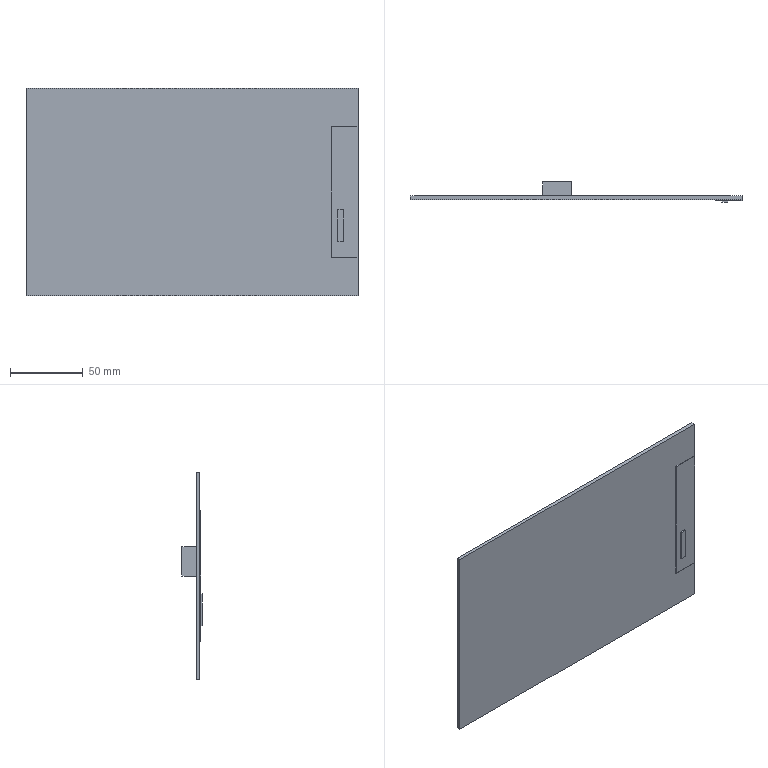Part | Creo | 1 solid | 22 faces | box 228.6 x 13.85 x 143 mm | volume 73471 mm3 | plane 22